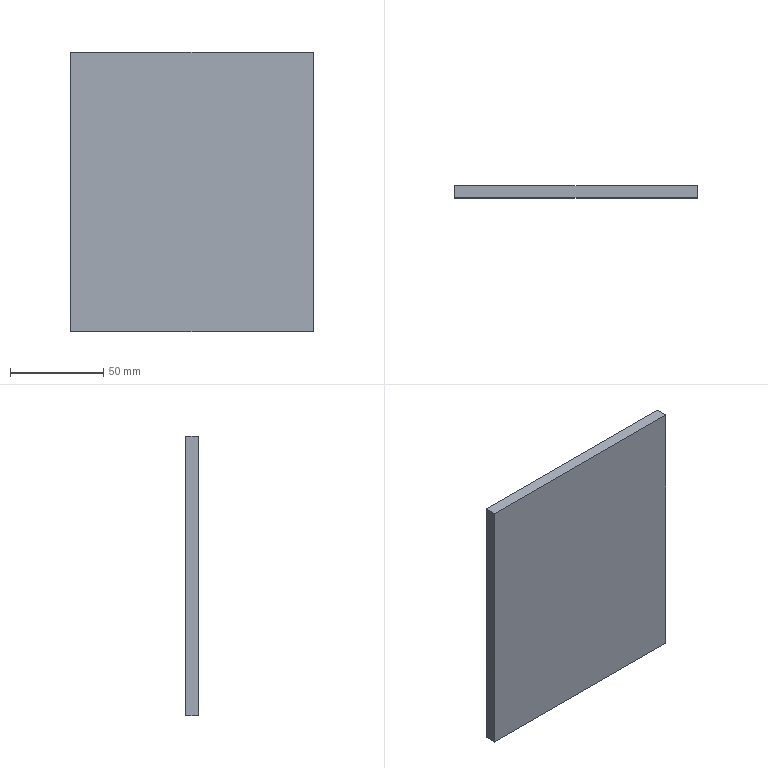Part | SolidWorks | features Extrusion 1 | 1 solid | 6 faces | box 130 x 6.5 x 150 mm | volume 126750 mm3 | plane 6
STEP:
#1=CARTESIAN_POINT('',(65.,0.,75.));
#2=VERTEX_POINT('',#1);
#3=CARTESIAN_POINT('',(65.,0.,-75.));
#4=VERTEX_POINT('',#3);
#5=CARTESIAN_POINT('',(65.,0.,75.));
#6=DIRECTION('',(0.,0.,-1.));
#7=VECTOR('',#6,1000.);
#8=LINE('',#5,#7);
#9=EDGE_CURVE('',#2,#4,#8,.T.);
#10=ORIENTED_EDGE('',*,*,#9,.T.);
#11=CARTESIAN_POINT('',(65.,6.5,-75.));
#12=VERTEX_POINT('',#11);
#13=CARTESIAN_POINT('',(65.,6.5,-75.));
#14=DIRECTION('',(0.,-1.,0.));
#15=VECTOR('',#14,1000.);
#16=LINE('',#13,#15);
#17=EDGE_CURVE('',#12,#4,#16,.T.);
#18=ORIENTED_EDGE('',*,*,#17,.F.);
#19=CARTESIAN_POINT('',(65.,6.5,75.));
#20=VERTEX_POINT('',#19);
#21=CARTESIAN_POINT('',(65.,6.5,75.));
#22=DIRECTION('',(0.,0.,-1.));
#23=VECTOR('',#22,1000.);
#24=LINE('',#21,#23);
#25=EDGE_CURVE('',#20,#12,#24,.T.);
#26=ORIENTED_EDGE('',*,*,#25,.F.);
#27=CARTESIAN_POINT('',(65.,6.5,75.));
#28=DIRECTION('',(0.,-1.,0.));
#29=VECTOR('',#28,1000.);
#30=LINE('',#27,#29);
#31=EDGE_CURVE('',#20,#2,#30,.T.);
#32=ORIENTED_EDGE('',*,*,#31,.T.);
#33=EDGE_LOOP('',(#10,#18,#26,#32));
#34=FACE_OUTER_BOUND('',#33,.T.);
#35=CARTESIAN_POINT('',(65.,6.5,75.));
#36=DIRECTION('',(-1.,0.,0.));
#37=DIRECTION('',(0.,0.,1.));
#38=AXIS2_PLACEMENT_3D('',#35,#36,#37);
#39=PLANE('',#38);
#40=ADVANCED_FACE('',(#34),#39,.F.);
#41=CARTESIAN_POINT('',(-65.,0.,-75.));
#42=VERTEX_POINT('',#41);
#43=CARTESIAN_POINT('',(-65.,0.,-75.));
#44=DIRECTION('',(-1.,0.,0.));
#45=VECTOR('',#44,1000.);
#46=LINE('',#43,#45);
#47=EDGE_CURVE('',#4,#42,#46,.T.);
#48=ORIENTED_EDGE('',*,*,#47,.T.);
#49=CARTESIAN_POINT('',(-65.,6.5,-75.));
#50=VERTEX_POINT('',#49);
#51=CARTESIAN_POINT('',(-65.,6.5,-75.));
#52=DIRECTION('',(0.,-1.,0.));
#53=VECTOR('',#52,1000.);
#54=LINE('',#51,#53);
#55=EDGE_CURVE('',#50,#42,#54,.T.);
#56=ORIENTED_EDGE('',*,*,#55,.F.);
#57=CARTESIAN_POINT('',(-65.,6.5,-75.));
#58=DIRECTION('',(-1.,0.,0.));
#59=VECTOR('',#58,1000.);
#60=LINE('',#57,#59);
#61=EDGE_CURVE('',#12,#50,#60,.T.);
#62=ORIENTED_EDGE('',*,*,#61,.F.);
#63=ORIENTED_EDGE('',*,*,#17,.T.);
#64=EDGE_LOOP('',(#48,#56,#62,#63));
#65=FACE_OUTER_BOUND('',#64,.T.);
#66=CARTESIAN_POINT('',(-65.,6.5,-75.));
#67=DIRECTION('',(0.,0.,1.));
#68=DIRECTION('',(1.,0.,0.));
#69=AXIS2_PLACEMENT_3D('',#66,#67,#68);
#70=PLANE('',#69);
#71=ADVANCED_FACE('',(#65),#70,.F.);
#72=CARTESIAN_POINT('',(-65.,0.,75.));
#73=VERTEX_POINT('',#72);
#74=CARTESIAN_POINT('',(-65.,0.,75.));
#75=DIRECTION('',(0.,0.,1.));
#76=VECTOR('',#75,1000.);
#77=LINE('',#74,#76);
#78=EDGE_CURVE('',#42,#73,#77,.T.);
#79=ORIENTED_EDGE('',*,*,#78,.T.);
#80=CARTESIAN_POINT('',(-65.,6.5,75.));
#81=VERTEX_POINT('',#80);
#82=CARTESIAN_POINT('',(-65.,6.5,75.));
#83=DIRECTION('',(0.,-1.,0.));
#84=VECTOR('',#83,1000.);
#85=LINE('',#82,#84);
#86=EDGE_CURVE('',#81,#73,#85,.T.);
#87=ORIENTED_EDGE('',*,*,#86,.F.);
#88=CARTESIAN_POINT('',(-65.,6.5,75.));
#89=DIRECTION('',(0.,0.,1.));
#90=VECTOR('',#89,1000.);
#91=LINE('',#88,#90);
#92=EDGE_CURVE('',#50,#81,#91,.T.);
#93=ORIENTED_EDGE('',*,*,#92,.F.);
#94=ORIENTED_EDGE('',*,*,#55,.T.);
#95=EDGE_LOOP('',(#79,#87,#93,#94));
#96=FACE_OUTER_BOUND('',#95,.T.);
#97=CARTESIAN_POINT('',(-65.,6.5,75.));
#98=DIRECTION('',(1.,0.,0.));
#99=DIRECTION('',(0.,0.,-1.));
#100=AXIS2_PLACEMENT_3D('',#97,#98,#99);
#101=PLANE('',#100);
#102=ADVANCED_FACE('',(#96),#101,.F.);
#103=CARTESIAN_POINT('',(-65.,0.,75.));
#104=DIRECTION('',(1.,0.,0.));
#105=VECTOR('',#104,1000.);
#106=LINE('',#103,#105);
#107=EDGE_CURVE('',#73,#2,#106,.T.);
#108=ORIENTED_EDGE('',*,*,#107,.T.);
#109=ORIENTED_EDGE('',*,*,#31,.F.);
#110=CARTESIAN_POINT('',(-65.,6.5,75.));
#111=DIRECTION('',(1.,0.,0.));
#112=VECTOR('',#111,1000.);
#113=LINE('',#110,#112);
#114=EDGE_CURVE('',#81,#20,#113,.T.);
#115=ORIENTED_EDGE('',*,*,#114,.F.);
#116=ORIENTED_EDGE('',*,*,#86,.T.);
#117=EDGE_LOOP('',(#108,#109,#115,#116));
#118=FACE_OUTER_BOUND('',#117,.T.);
#119=CARTESIAN_POINT('',(-65.,6.5,75.));
#120=DIRECTION('',(0.,0.,-1.));
#121=DIRECTION('',(-1.,0.,0.));
#122=AXIS2_PLACEMENT_3D('',#119,#120,#121);
#123=PLANE('',#122);
#124=ADVANCED_FACE('',(#118),#123,.F.);
#125=ORIENTED_EDGE('',*,*,#25,.T.);
#126=ORIENTED_EDGE('',*,*,#61,.T.);
#127=ORIENTED_EDGE('',*,*,#92,.T.);
#128=ORIENTED_EDGE('',*,*,#114,.T.);
#129=EDGE_LOOP('',(#125,#126,#127,#128));
#130=FACE_OUTER_BOUND('',#129,.T.);
#131=CARTESIAN_POINT('',(0.,6.5,0.));
#132=DIRECTION('',(0.,-1.,0.));
#133=DIRECTION('',(0.,0.,-1.));
#134=AXIS2_PLACEMENT_3D('',#131,#132,#133);
#135=PLANE('',#134);
#136=ADVANCED_FACE('',(#130),#135,.F.);
#137=ORIENTED_EDGE('',*,*,#9,.F.);
#138=ORIENTED_EDGE('',*,*,#107,.F.);
#139=ORIENTED_EDGE('',*,*,#78,.F.);
#140=ORIENTED_EDGE('',*,*,#47,.F.);
#141=EDGE_LOOP('',(#137,#138,#139,#140));
#142=FACE_OUTER_BOUND('',#141,.T.);
#143=CARTESIAN_POINT('',(0.,0.,0.));
#144=DIRECTION('',(0.,-1.,0.));
#145=DIRECTION('',(0.,0.,-1.));
#146=AXIS2_PLACEMENT_3D('',#143,#144,#145);
#147=PLANE('',#146);
#148=ADVANCED_FACE('',(#142),#147,.T.);
#149=CLOSED_SHELL('',(#40,#71,#102,#124,#136,#148));
#150=MANIFOLD_SOLID_BREP('',#149);
#151=CARTESIAN_POINT('',(0.,0.,0.));
#152=DIRECTION('',(0.,0.,1.));
#153=DIRECTION('',(1.,0.,0.));
#154=AXIS2_PLACEMENT_3D('',#151,#152,#153);
#155=(LENGTH_UNIT()NAMED_UNIT(*)SI_UNIT(.MILLI.,.METRE.));
#156=UNCERTAINTY_MEASURE_WITH_UNIT(LENGTH_MEASURE(0.00001),#155,'','');
#157=(NAMED_UNIT(*)PLANE_ANGLE_UNIT()SI_UNIT($,.RADIAN.));
#158=(NAMED_UNIT(*)SI_UNIT($,.STERADIAN.)SOLID_ANGLE_UNIT());
#159=(GEOMETRIC_REPRESENTATION_CONTEXT(3)GLOBAL_UNCERTAINTY_ASSIGNED_CONTEXT((#156))GLOBAL_UNIT_ASSIGNED_CONTEXT((#155,#157,#158))REPRESENTATION_CONTEXT('',''));
#160=ADVANCED_BREP_SHAPE_REPRESENTATION('',(#150,#154),#159);